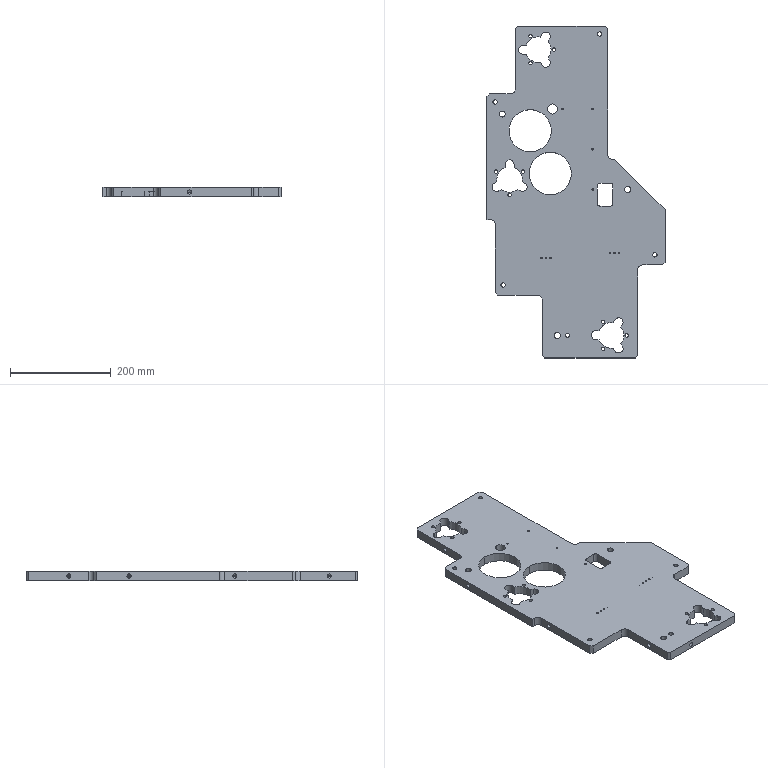NC program | NX | posted with a generic post | part box 354 x 660 x 18 mm
Lines 42 to 865 of 43361:
(ZLEVEL_PROFILE , TOOL : D8C)
N76 T08 M6
N78 G54
N80 G17 G0 G90 X-315.203 Y87.193 S4000 M3
N82 G43 Z30. H8
N84 Z1.7
N86 G94 G1 X-315.332 Y86.951 Z1.686 F1000.
N88 X-315.481 Y86.678 Z1.669
N90 X-315.628 Y86.323 Z1.649
N92 X-315.717 Y86.025 Z1.633
N94 X-315.721 Y86.017 Z1.632
N96 X-315.811 Y85.714 Z1.616
N98 X-315.919 Y85.036 Z1.58
N100 X-315.926 Y84.721 Z1.563
N102 X-315.934 Y84.411 Z1.547
N104 X-315.894 Y83.955 Z1.523
N106 X-315.811 Y83.504 Z1.499
N108 X-315.721 Y83.208 Z1.483
N110 X-315.681 Y83.081 Z1.476
N112 X-315.596 Y82.804 Z1.461
N114 X-315.465 Y82.499 Z1.443
N116 X-315.323 Y82.247 Z1.428
N118 X-314.989 Y81.708 Z1.395
N120 X-314.625 Y81.271 Z1.365
N122 X-314.42 Y81.044 Z1.349
N124 X-313.946 Y80.64 Z1.316
N126 X-313.679 Y80.469 Z1.3
N128 X-313.461 Y80.33 Z1.286
N130 X-313.463 Y80.327
N132 X-308.138 Y77.253 Z0.964
N134 X-307.891 Y77.111 Z0.949
N136 X-307.33 Y76.653 Z0.911
N138 X-306.858 Y76.104 Z0.873
N140 X-306.492 Y75.48 Z0.835
N142 X-306.242 Y74.8 Z0.797
N144 X-306.117 Y74.087 Z0.759
N146 X-306.12 Y73.363 Z0.721
N148 X-306.167 Y73.082 Z0.706
N150 X-306.273 Y72.404 Z0.67
N152 X-306.382 Y71.353 Z0.615
N154 X-306.444 Y70.298 Z0.56
N156 X-306.449 Y69.612 Z0.524
N158 X-306.445 Y68.931 Z0.488
N160 X-306.378 Y67.806 Z0.429
N162 X-306.256 Y66.685 Z0.37
N164 X-306.146 Y66.012 Z0.334
N166 X-306.143
N168 X-306.029 Y65.356 Z0.299
N170 X-305.915 Y64.834 Z0.271
N172 X-305.744 Y64.183 Z0.236
N174 X-305.673 Y63.879 Z0.219
N176 X-305.58 Y63.581 Z0.203
N178 X-305.487 Y63.285 Z0.187
N180 X-305.347 Y62.837 Z0.162
N182 X-305.35 Y62.828
N184 X-305.345 Y62.829
N186 X-305.305 Y62.696 Z0.154
N188 X-304.948 Y61.738 Z0.101
N190 X-304.951 Y61.732 Z0.1
N192 X-304.946 Y61.733
N194 X-304.549 Y60.8 F2500.
N196 X-304.195 Y60.044
N198 X-304.145 Y59.956
N200 X-303.751 Y59.207
N202 X-303.566 Y58.883
N204 G3 X-302.951 Y57.883 R13.689
N206 X-302.414 Y57.099 R14.8
N208 G1 X-302.149 Y56.737
N210 G3 X-301.638 Y56.085 R9.006
N212 X-300.947 Y55.275 R13.979
N214 X-299.794 Y54.088 R20.277
N216 X-298.914 Y53.295 R18.733
N218 G1 X-298.575 Y53.008
N220 X-297.741 Y52.352
N222 X-296.953 Y51.807
N224 G3 X-296.14 Y51.289 R12.608
N226 X-295.457 Y50.889 R6.805
N228 X-293.884 Y50.093 R16.957
N230 G1 X-293.643 Y49.967
N232 X-292.938 Y49.691
N234 X-292.463 Y49.497
N236 G2 X-289.95 Y45.751 R4.049
N238 G1 Y39.6
N240 G3 X-289.786 Y38.377 R5.145
N242 X-289.385 Y37.327 R4.407
N244 X-288.84 Y36.499 R5.438
N246 X-288.484 Y36.107 R2.892
N248 G1 X-288.478 Y36.1
N250 G3 X-287.61 Y35.408 R5.05
N252 G1 X-287.414 Y35.299
N254 G3 X-286.5 Y34.902 R4.509
N256 G1 X-286.489 Y34.895
N258 G3 X-283.504 Y34.898 R4.886
N260 G1 X-283.497 Y34.902
N262 G3 X-282.768 Y35.201 R4.285
N264 G1 X-282.572 Y35.303
N266 G3 X-281.522 Y36.096 R4.826
N268 G1 X-281.514 Y36.106
N270 G3 X-280.605 Y37.341 R4.982
N272 X-280.245 Y38.241 R5.914
N274 G1 X-280.209 Y38.39
N276 G3 X-280.052 Y39.6 R5.341
N278 G1 X-280.05
N280 Y45.756
N282 G2 X-277.425 Y49.542 R4.046
N284 G1 X-277.061 Y49.689
N286 X-276.448 Y49.934
N288 X-275.222 Y50.516
N290 X-274.216 Y51.069
N292 X-273.503 Y51.509
N294 G3 X-272.633 Y52.093 R13.692
N296 X-271.834 Y52.686 R11.162
N298 X-271.094 Y53.287 R12.577
N300 G1 X-270.87 Y53.482
N302 G3 X-267.85 Y56.737 R21.15
N304 G1 X-267.737 Y56.892
N306 X-267.351 Y57.421
N308 X-267.044 Y57.891
N310 G3 X-266.251 Y59.2 R19.575
N312 G1 X-266.246 Y59.199
N314 X-265.854 Y59.956
N316 X-265.684 Y60.268
N318 X-265.45 Y60.801
N320 X-265.412 Y60.886
N322 X-265.071 Y61.686
N324 X-265.051 Y61.74
N326 X-264.708 Y62.658
N328 X-264.652 Y62.838
N330 G3 X-264.253 Y64.19 R18.089
N332 X-263.857 Y66.001 R21.717
N334 G1 X-263.855 Y66.007
N336 G3 X-263.696 Y72.079 R21.95
N338 G1 X-263.849 Y73.202
N340 G2 X-261.866 Y77.251 R4.042
N342 G1 X-256.373 Y80.422
N344 X-256.312 Y80.474
N346 G3 X-255.145 Y81.532 R4.956
N348 G1 X-255.075 Y81.628
N350 G3 X-254.279 Y83.2 R5.039
N352 X-254.279 Y86.015 R4.902
N354 G1 X-254.283 Y86.019
N356 G3 X-254.677 Y86.974 R4.82
N358 G1 X-254.682 Y86.987
N360 G3 X-255.076 Y87.593 R5.023
N362 G1 X-255.081 Y87.594
N364 G3 X-255.3 Y87.871 R5.265
N366 G1 X-255.483 Y88.064
N368 G3 X-256.508 Y88.868 R4.695
N370 G1 X-256.728 Y88.989
N372 G3 X-257.377 Y89.273 R3.959
N374 X-260.678 Y89.274 R4.998
N376 G1 X-260.68 Y89.269
N378 G3 X-261.486 Y88.898 R5.067
N380 G1 X-261.487 Y88.901
N382 X-266.53 Y85.989
N384 X-266.88 Y85.794
N386 G2 X-271.38 Y86.182 R4.032
N388 G1 X-271.753 Y86.47
N390 X-272.302 Y86.905
N392 X-273.381 Y87.638
N394 X-274.293 Y88.197
N396 X-275.376 Y88.782
N398 X-275.578 Y88.874
N400 X-275.825 Y88.99
N402 G3 X-280.03 Y90.471 R20.692
N404 X-282.157 Y90.868 R23.522
N406 G1 X-282.164 Y90.872
N408 G3 X-282.971 Y90.956 R58.63
N410 X-287.321 Y90.926 R20.955
N412 G1 X-287.822 Y90.87
N414 X-287.834 Y90.872
N416 X-287.835 Y90.868
N418 G3 X-289.975 Y90.468 R22.685
N420 X-294.192 Y88.983 R21.031
N422 G1 X-294.431 Y88.869
N424 X-294.574 Y88.801
N426 X-295.2 Y88.469
N428 G3 X-295.91 Y88.071 R11.94
N430 G1 X-296.631 Y87.63
N432 X-297.719 Y86.89
N434 X-298.563 Y86.224
N436 X-298.763 Y86.071
N438 G2 X-303.18 Y85.822 R4.05
N440 G1 X-308.513 Y88.901
N442 G3 X-312.526 Y89.305 R4.979
N444 G1 X-312.633 Y89.267
N446 G3 X-313.324 Y88.963 R4.463
N448 G1 X-313.491 Y88.867
N450 G3 X-314.523 Y88.055 R4.659
N452 X-315.332 Y86.951 R4.692
N454 X-315.717 Y86.025 R4.823
N456 G1 X-315.721 Y86.017
N458 G3 X-315.926 Y84.721 R4.965
N460 X-315.721 Y83.208 R4.791
N462 G1 X-315.681 Y83.081
N464 G3 X-315.323 Y82.247 R4.196
N466 G1 X-314.989 Y81.708
N468 X-314.625 Y81.271
N470 G3 X-313.679 Y80.469 R4.668
N472 G1 X-313.461 Y80.33
N474 X-313.463 Y80.327
N476 X-308.138 Y77.253
N478 G2 X-306.167 Y73.082 R4.053
N480 G3 X-306.449 Y69.612 R23.545
N482 X-306.146 Y66.012 R23.225
N484 G1 X-306.143
N486 G3 X-305.744 Y64.183 R22.152
N488 X-305.58 Y63.581 R8.727
N490 G1 X-305.487 Y63.285
N492 X-305.347 Y62.837
N494 X-305.35 Y62.828
N496 X-305.345 Y62.829
N498 G3 X-305.257 Y62.566 R4.205
N500 G1 X-304.948 Y61.738
N502 X-304.951 Y61.732
N504 X-304.946 Y61.733
N506 X-304.951 Y61.732
N508 X-304.877 Y61.548 Z0.097
N510 X-304.802 Y61.365 Z0.093
N512 X-304.725 Y61.183 Z0.09
N514 X-304.647 Y61.002 Z0.086
N516 X-304.567 Y60.822 Z0.083
N518 X-304.485 Y60.642 Z0.079
N520 X-304.402 Y60.463 Z0.076
N522 X-304.317 Y60.284 Z0.072
N524 X-304.23 Y60.107 Z0.069
N526 X-304.142 Y59.93 Z0.066
N528 X-304.052 Y59.754 Z0.062
N530 X-303.96 Y59.579 Z0.059
N532 X-303.867 Y59.405 Z0.055
N534 X-303.772 Y59.232 Z0.052
N536 X-303.676 Y59.059 Z0.048
N538 X-303.578 Y58.888 Z0.045
N540 X-303.478 Y58.717 Z0.041
N542 X-303.377 Y58.547 Z0.038
N544 X-303.274 Y58.379 Z0.034
N546 X-303.17 Y58.211 Z0.031
N548 X-303.065 Y58.044 Z0.028
N550 X-302.957 Y57.878 Z0.024
N552 X-302.848 Y57.713 Z0.021
N554 X-302.738 Y57.549 Z0.017
N556 X-302.626 Y57.386 Z0.014
N558 X-302.513 Y57.225 Z0.01
N560 X-302.398 Y57.064 Z0.007
N562 X-302.282 Y56.904 Z0.003
N564 X-302.164 Y56.745 Z0.
N566 G3 X-292.571 Y49.54 R21.45
N568 G2 X-289.95 Y45.751 R4.05
N570 G1 Y39.61
N572 G3 X-285. Y34.66 R4.95
N574 X-280.05 Y39.61 R4.95
N576 G1 Y45.751
N578 G2 X-277.429 Y49.54 R4.05
N580 G3 X-263.834 Y73.088 R21.45
N582 G2 X-261.863 Y77.253 R4.05
N584 G1 X-256.544 Y80.323
N586 G3 X-254.732 Y87.085 R4.95
N588 X-261.494 Y88.897 R4.95
N590 G1 X-266.371 Y86.082
N592 X-266.551 Y85.977
N594 X-266.573 Y85.976
N596 G2 X-271.405 Y86.201 R4.05
N598 G3 X-298.166 Y86.544 R21.45
N600 G1 X-298.165 Y86.533
N602 X-298.444 Y86.318
N604 X-298.46 Y86.317
N606 G2 X-303.187 Y85.826 R4.05
N608 G1 X-308.506 Y88.897
N610 G3 X-315.268 Y87.085 R4.95
N612 X-313.456 Y80.323 R4.95
N614 G1 X-308.137 Y77.253
N616 G2 X-306.166 Y73.088 R4.05
N618 G3 X-304.951 Y61.732 R21.45
N620 G1 X-304.879 Y61.555 Z-0.003
N622 X-304.803 Y61.379 Z-0.007
N624 X-304.727 Y61.204 Z-0.01
N626 X-304.649 Y61.03 Z-0.013
N628 X-304.573 Y60.855 Z-0.017
N630 X-304.496 Y60.68 Z-0.02
N632 X-304.421 Y60.505 Z-0.023
N634 X-304.336 Y60.334 Z-0.027
N636 X-304.25 Y60.163 Z-0.03
N638 X-304.163 Y59.993 Z-0.033
N640 X-304.078 Y59.822 Z-0.037
N642 X-303.992 Y59.652 Z-0.04
N644 X-303.906 Y59.481 Z-0.043
N646 X-303.814 Y59.314 Z-0.047
N648 X-303.718 Y59.149 Z-0.05
N650 X-303.622 Y58.984 Z-0.053
N652 X-303.528 Y58.818 Z-0.057
N654 X-303.433 Y58.652 Z-0.06
N656 X-303.337 Y58.487 Z-0.063
N658 X-303.238 Y58.324 Z-0.067
N660 X-303.134 Y58.164 Z-0.07
N662 X-303.03 Y58.004 Z-0.073
N664 X-302.925 Y57.844 Z-0.077
N666 X-302.82 Y57.684 Z-0.08
N668 X-302.717 Y57.524 Z-0.083
N670 X-302.61 Y57.365 Z-0.087
N672 X-302.496 Y57.212 Z-0.09
N674 X-302.384 Y57.057 Z-0.093
N676 X-302.271 Y56.904 Z-0.097
N678 X-302.164 Y56.745 Z-0.1
N680 G3 X-292.571 Y49.54 R21.45
N682 G2 X-289.95 Y45.751 R4.05
N684 G1 Y39.61
N686 G3 X-285. Y34.66 R4.95
N688 X-280.05 Y39.61 R4.95
N690 G1 Y45.751
N692 G2 X-277.429 Y49.54 R4.05
N694 G3 X-263.834 Y73.088 R21.45
N696 G2 X-261.863 Y77.253 R4.05
N698 G1 X-256.544 Y80.323
N700 G3 X-254.732 Y87.085 R4.95
N702 X-261.494 Y88.897 R4.95
N704 G1 X-266.371 Y86.082
N706 X-266.551 Y85.977
N708 X-266.573 Y85.976
N710 G2 X-271.405 Y86.201 R4.05
N712 G3 X-298.166 Y86.544 R21.45
N714 G1 X-298.165 Y86.533
N716 X-298.444 Y86.318
N718 X-298.46 Y86.317
N720 G2 X-303.187 Y85.826 R4.05
N722 G1 X-308.506 Y88.897
N724 G3 X-315.268 Y87.085 R4.95
N726 X-313.456 Y80.323 R4.95
N728 G1 X-308.137 Y77.253
N730 G2 X-306.166 Y73.088 R4.05
N732 G3 X-304.951 Y61.732 R21.45
N734 G1 X-304.879 Y61.555 Z-0.103
N736 X-304.803 Y61.379 Z-0.107
N738 X-304.727 Y61.204 Z-0.11
N740 X-304.649 Y61.03 Z-0.113
N742 X-304.573 Y60.855 Z-0.117
N744 X-304.496 Y60.68 Z-0.12
N746 X-304.421 Y60.505 Z-0.123
N748 X-304.336 Y60.334 Z-0.127
N750 X-304.25 Y60.163 Z-0.13
N752 X-304.163 Y59.993 Z-0.133
N754 X-304.078 Y59.822 Z-0.137
N756 X-303.992 Y59.652 Z-0.14
N758 X-303.906 Y59.481 Z-0.143
N760 X-303.814 Y59.314 Z-0.147
N762 X-303.718 Y59.149 Z-0.15
N764 X-303.622 Y58.984 Z-0.153
N766 X-303.528 Y58.818 Z-0.157
N768 X-303.433 Y58.652 Z-0.16
N770 X-303.337 Y58.487 Z-0.163
N772 X-303.238 Y58.324 Z-0.167
N774 X-303.134 Y58.164 Z-0.17
N776 X-303.03 Y58.004 Z-0.173
N778 X-302.925 Y57.844 Z-0.177
N780 X-302.82 Y57.684 Z-0.18
N782 X-302.717 Y57.524 Z-0.183
N784 X-302.61 Y57.365 Z-0.187
N786 X-302.496 Y57.212 Z-0.19
N788 X-302.384 Y57.057 Z-0.193
N790 X-302.271 Y56.904 Z-0.197
N792 X-302.164 Y56.745 Z-0.2
N794 G3 X-292.571 Y49.54 R21.45
N796 G2 X-289.95 Y45.751 R4.05
N798 G1 Y39.61
N800 G3 X-285. Y34.66 R4.95
N802 X-280.05 Y39.61 R4.95
N804 G1 Y45.751
N806 G2 X-277.429 Y49.54 R4.05
N808 G3 X-263.834 Y73.088 R21.45
N810 G2 X-261.863 Y77.253 R4.05
N812 G1 X-256.544 Y80.323
N814 G3 X-254.732 Y87.085 R4.95
N816 X-261.494 Y88.897 R4.95
N818 G1 X-266.371 Y86.082
N820 X-266.551 Y85.977
N822 X-266.573 Y85.976
N824 G2 X-271.405 Y86.201 R4.05
N826 G3 X-298.166 Y86.544 R21.45
N828 G1 X-298.165 Y86.533
N830 X-298.444 Y86.318
N832 X-298.46 Y86.317
N834 G2 X-303.187 Y85.826 R4.05
N836 G1 X-308.506 Y88.897
N838 G3 X-315.268 Y87.085 R4.95
N840 X-313.456 Y80.323 R4.95
N842 G1 X-308.137 Y77.253
N844 G2 X-306.166 Y73.088 R4.05
N846 G3 X-304.951 Y61.732 R21.45
N848 G1 X-304.879 Y61.555 Z-0.203
N850 X-304.803 Y61.379 Z-0.207
N852 X-304.727 Y61.204 Z-0.21
N854 X-304.649 Y61.03 Z-0.213
N856 X-304.573 Y60.855 Z-0.217
N858 X-304.496 Y60.68 Z-0.22
N860 X-304.421 Y60.505 Z-0.223
N862 X-304.336 Y60.334 Z-0.227
N864 X-304.25 Y60.163 Z-0.23
N866 X-304.163 Y59.993 Z-0.233
N868 X-304.078 Y59.822 Z-0.237
N870 X-303.992 Y59.652 Z-0.24
N872 X-303.906 Y59.481 Z-0.243
N874 X-303.814 Y59.314 Z-0.247
N876 X-303.718 Y59.149 Z-0.25
N878 X-303.622 Y58.984 Z-0.253
N880 X-303.528 Y58.818 Z-0.257
N882 X-303.433 Y58.652 Z-0.26
N884 X-303.337 Y58.487 Z-0.263
N886 X-303.238 Y58.324 Z-0.267
N888 X-303.134 Y58.164 Z-0.27
N890 X-303.03 Y58.004 Z-0.273
N892 X-302.925 Y57.844 Z-0.277
N894 X-302.82 Y57.684 Z-0.28
N896 X-302.717 Y57.524 Z-0.283
N898 X-302.61 Y57.365 Z-0.287
N900 X-302.496 Y57.212 Z-0.29
N902 X-302.384 Y57.057 Z-0.293
N904 X-302.271 Y56.904 Z-0.297
N906 X-302.164 Y56.745 Z-0.3
N908 G3 X-292.571 Y49.54 R21.45
N910 G2 X-289.95 Y45.751 R4.05
N912 G1 Y39.61
N914 G3 X-285. Y34.66 R4.95
N916 X-280.05 Y39.61 R4.95
N918 G1 Y45.751
N920 G2 X-277.429 Y49.54 R4.05
N922 G3 X-263.834 Y73.088 R21.45
N924 G2 X-261.863 Y77.253 R4.05
N926 G1 X-256.544 Y80.323
N928 G3 X-254.732 Y87.085 R4.95
N930 X-261.494 Y88.897 R4.95
N932 G1 X-266.371 Y86.082
N934 X-266.551 Y85.977
N936 X-266.573 Y85.976
N938 G2 X-271.405 Y86.201 R4.05
N940 G3 X-298.166 Y86.544 R21.45
N942 G1 X-298.165 Y86.533
N944 X-298.444 Y86.318
N946 X-298.46 Y86.317
N948 G2 X-303.187 Y85.826 R4.05
N950 G1 X-308.506 Y88.897
N952 G3 X-315.268 Y87.085 R4.95
N954 X-313.456 Y80.323 R4.95
N956 G1 X-308.137 Y77.253
N958 G2 X-306.166 Y73.088 R4.05
N960 G3 X-304.951 Y61.732 R21.45
N962 G1 X-304.879 Y61.555 Z-0.303
N964 X-304.803 Y61.379 Z-0.307
N966 X-304.727 Y61.204 Z-0.31
N968 X-304.649 Y61.03 Z-0.313
N970 X-304.573 Y60.855 Z-0.317
N972 X-304.496 Y60.68 Z-0.32
N974 X-304.421 Y60.505 Z-0.323
N976 X-304.336 Y60.334 Z-0.327
N978 X-304.25 Y60.163 Z-0.33
N980 X-304.163 Y59.993 Z-0.333
N982 X-304.078 Y59.822 Z-0.337
N984 X-303.992 Y59.652 Z-0.34
N986 X-303.906 Y59.481 Z-0.343
N988 X-303.814 Y59.314 Z-0.347
N990 X-303.718 Y59.149 Z-0.35
N992 X-303.622 Y58.984 Z-0.353
N994 X-303.528 Y58.818 Z-0.357
N996 X-303.433 Y58.652 Z-0.36
N998 X-303.337 Y58.487 Z-0.363
N1000 X-303.238 Y58.324 Z-0.367
N1002 X-303.134 Y58.164 Z-0.37
N1004 X-303.03 Y58.004 Z-0.373
N1006 X-302.925 Y57.844 Z-0.377
N1008 X-302.82 Y57.684 Z-0.38
N1010 X-302.717 Y57.524 Z-0.383
N1012 X-302.61 Y57.365 Z-0.387
N1014 X-302.496 Y57.212 Z-0.39
N1016 X-302.384 Y57.057 Z-0.393
N1018 X-302.271 Y56.904 Z-0.397
N1020 X-302.164 Y56.745 Z-0.4
N1022 G3 X-292.571 Y49.54 R21.45
N1024 G2 X-289.95 Y45.751 R4.05
N1026 G1 Y39.61
N1028 G3 X-285. Y34.66 R4.95
N1030 X-280.05 Y39.61 R4.95
N1032 G1 Y45.751
N1034 G2 X-277.429 Y49.54 R4.05
N1036 G3 X-263.834 Y73.088 R21.45
N1038 G2 X-261.863 Y77.253 R4.05
N1040 G1 X-256.544 Y80.323
N1042 G3 X-254.732 Y87.085 R4.95
N1044 X-261.494 Y88.897 R4.95
N1046 G1 X-266.371 Y86.082
N1048 X-266.551 Y85.977
N1050 X-266.573 Y85.976
N1052 G2 X-271.405 Y86.201 R4.05
N1054 G3 X-298.166 Y86.544 R21.45
N1056 G1 X-298.165 Y86.533
N1058 X-298.444 Y86.318
N1060 X-298.46 Y86.317
N1062 G2 X-303.187 Y85.826 R4.05
N1064 G1 X-308.506 Y88.897
N1066 G3 X-315.268 Y87.085 R4.95
N1068 X-313.456 Y80.323 R4.95
N1070 G1 X-308.137 Y77.253
N1072 G2 X-306.166 Y73.088 R4.05
N1074 G3 X-304.951 Y61.732 R21.45
N1076 G1 X-304.879 Y61.555 Z-0.403
N1078 X-304.803 Y61.379 Z-0.407
N1080 X-304.727 Y61.204 Z-0.41
N1082 X-304.649 Y61.03 Z-0.413
N1084 X-304.573 Y60.855 Z-0.417
N1086 X-304.496 Y60.68 Z-0.42
N1088 X-304.421 Y60.505 Z-0.423
N1090 X-304.336 Y60.334 Z-0.427
N1092 X-304.25 Y60.163 Z-0.43
N1094 X-304.163 Y59.993 Z-0.433
N1096 X-304.078 Y59.822 Z-0.437
N1098 X-303.992 Y59.652 Z-0.44
N1100 X-303.906 Y59.481 Z-0.443
N1102 X-303.814 Y59.314 Z-0.447
N1104 X-303.718 Y59.149 Z-0.45
N1106 X-303.622 Y58.984 Z-0.453
N1108 X-303.528 Y58.818 Z-0.457
N1110 X-303.433 Y58.652 Z-0.46
N1112 X-303.337 Y58.487 Z-0.463
N1114 X-303.238 Y58.324 Z-0.467
N1116 X-303.134 Y58.164 Z-0.47
N1118 X-303.03 Y58.004 Z-0.473
N1120 X-302.925 Y57.844 Z-0.477
N1122 X-302.82 Y57.684 Z-0.48
N1124 X-302.717 Y57.524 Z-0.483
N1126 X-302.61 Y57.365 Z-0.487
N1128 X-302.496 Y57.212 Z-0.49
N1130 X-302.384 Y57.057 Z-0.493
N1132 X-302.271 Y56.904 Z-0.497
N1134 X-302.164 Y56.745 Z-0.5
N1136 G3 X-292.571 Y49.54 R21.45
N1138 G2 X-289.95 Y45.751 R4.05
N1140 G1 Y39.61
N1142 G3 X-285. Y34.66 R4.95
N1144 X-280.05 Y39.61 R4.95
N1146 G1 Y45.751
N1148 G2 X-277.429 Y49.54 R4.05
N1150 G3 X-263.834 Y73.088 R21.45
N1152 G2 X-261.863 Y77.253 R4.05
N1154 G1 X-256.544 Y80.323
N1156 G3 X-254.732 Y87.085 R4.95
N1158 X-261.494 Y88.897 R4.95
N1160 G1 X-266.371 Y86.082
N1162 X-266.551 Y85.977
N1164 X-266.573 Y85.976
N1166 G2 X-271.405 Y86.201 R4.05
N1168 G3 X-298.166 Y86.544 R21.45
N1170 G1 X-298.165 Y86.533
N1172 X-298.444 Y86.318
N1174 X-298.46 Y86.317
N1176 G2 X-303.187 Y85.826 R4.05
N1178 G1 X-308.506 Y88.897
N1180 G3 X-315.268 Y87.085 R4.95
N1182 X-313.456 Y80.323 R4.95
N1184 G1 X-308.137 Y77.253
N1186 G2 X-306.166 Y73.088 R4.05
N1188 G3 X-304.951 Y61.732 R21.45
N1190 G1 X-304.879 Y61.555 Z-0.503
N1192 X-304.803 Y61.379 Z-0.507
N1194 X-304.727 Y61.204 Z-0.51
N1196 X-304.649 Y61.03 Z-0.513
N1198 X-304.573 Y60.855 Z-0.517
N1200 X-304.496 Y60.68 Z-0.52
N1202 X-304.421 Y60.505 Z-0.523
N1204 X-304.336 Y60.334 Z-0.527
N1206 X-304.25 Y60.163 Z-0.53
N1208 X-304.163 Y59.993 Z-0.533
N1210 X-304.078 Y59.822 Z-0.537
N1212 X-303.992 Y59.652 Z-0.54
N1214 X-303.906 Y59.481 Z-0.543
N1216 X-303.814 Y59.314 Z-0.547
N1218 X-303.718 Y59.149 Z-0.55
N1220 X-303.622 Y58.984 Z-0.553
N1222 X-303.528 Y58.818 Z-0.557
N1224 X-303.433 Y58.652 Z-0.56
N1226 X-303.337 Y58.487 Z-0.563
N1228 X-303.238 Y58.324 Z-0.567
N1230 X-303.134 Y58.164 Z-0.57
N1232 X-303.03 Y58.004 Z-0.573
N1234 X-302.925 Y57.844 Z-0.577
N1236 X-302.82 Y57.684 Z-0.58
N1238 X-302.717 Y57.524 Z-0.583
N1240 X-302.61 Y57.365 Z-0.587
N1242 X-302.496 Y57.212 Z-0.59
N1244 X-302.384 Y57.057 Z-0.593
N1246 X-302.271 Y56.904 Z-0.597
N1248 X-302.164 Y56.745 Z-0.6
N1250 G3 X-292.571 Y49.54 R21.45
N1252 G2 X-289.95 Y45.751 R4.05
N1254 G1 Y39.61
N1256 G3 X-285. Y34.66 R4.95
N1258 X-280.05 Y39.61 R4.95
N1260 G1 Y45.751
N1262 G2 X-277.429 Y49.54 R4.05
N1264 G3 X-263.834 Y73.088 R21.45
N1266 G2 X-261.863 Y77.253 R4.05
N1268 G1 X-256.544 Y80.323
N1270 G3 X-254.732 Y87.085 R4.95
N1272 X-261.494 Y88.897 R4.95
N1274 G1 X-266.371 Y86.082
N1276 X-266.551 Y85.977
N1278 X-266.573 Y85.976
N1280 G2 X-271.405 Y86.201 R4.05
N1282 G3 X-298.166 Y86.544 R21.45
N1284 G1 X-298.165 Y86.533
N1286 X-298.444 Y86.318
N1288 X-298.46 Y86.317
N1290 G2 X-303.187 Y85.826 R4.05
N1292 G1 X-308.506 Y88.897
N1294 G3 X-315.268 Y87.085 R4.95
N1296 X-313.456 Y80.323 R4.95
N1298 G1 X-308.137 Y77.253
N1300 G2 X-306.166 Y73.088 R4.05
N1302 G3 X-304.951 Y61.732 R21.45
N1304 G1 X-304.879 Y61.555 Z-0.603
N1306 X-304.803 Y61.379 Z-0.607
N1308 X-304.727 Y61.204 Z-0.61
N1310 X-304.649 Y61.03 Z-0.613
N1312 X-304.573 Y60.855 Z-0.617
N1314 X-304.496 Y60.68 Z-0.62
N1316 X-304.421 Y60.505 Z-0.623
N1318 X-304.336 Y60.334 Z-0.627
N1320 X-304.25 Y60.163 Z-0.63
N1322 X-304.163 Y59.993 Z-0.633
N1324 X-304.078 Y59.822 Z-0.637
N1326 X-303.992 Y59.652 Z-0.64
N1328 X-303.906 Y59.481 Z-0.643
N1330 X-303.814 Y59.314 Z-0.647
N1332 X-303.718 Y59.149 Z-0.65
N1334 X-303.622 Y58.984 Z-0.653
N1336 X-303.528 Y58.818 Z-0.657
N1338 X-303.433 Y58.652 Z-0.66
N1340 X-303.337 Y58.487 Z-0.663
N1342 X-303.238 Y58.324 Z-0.667
N1344 X-303.134 Y58.164 Z-0.67
N1346 X-303.03 Y58.004 Z-0.673
N1348 X-302.925 Y57.844 Z-0.677
N1350 X-302.82 Y57.684 Z-0.68
N1352 X-302.717 Y57.524 Z-0.683
N1354 X-302.61 Y57.365 Z-0.687
N1356 X-302.496 Y57.212 Z-0.69
N1358 X-302.384 Y57.057 Z-0.693
N1360 X-302.271 Y56.904 Z-0.697
N1362 X-302.164 Y56.745 Z-0.7
N1364 G3 X-292.571 Y49.54 R21.45
N1366 G2 X-289.95 Y45.751 R4.05
N1368 G1 Y39.61
N1370 G3 X-285. Y34.66 R4.95
N1372 X-280.05 Y39.61 R4.95
N1374 G1 Y45.751
N1376 G2 X-277.429 Y49.54 R4.05
N1378 G3 X-263.834 Y73.088 R21.45
N1380 G2 X-261.863 Y77.253 R4.05
N1382 G1 X-256.544 Y80.323
N1384 G3 X-254.732 Y87.085 R4.95
N1386 X-261.494 Y88.897 R4.95
N1388 G1 X-266.371 Y86.082
N1390 X-266.551 Y85.977
N1392 X-266.573 Y85.976
N1394 G2 X-271.405 Y86.201 R4.05
N1396 G3 X-298.166 Y86.544 R21.45
N1398 G1 X-298.165 Y86.533
N1400 X-298.444 Y86.318
N1402 X-298.46 Y86.317
N1404 G2 X-303.187 Y85.826 R4.05
N1406 G1 X-308.506 Y88.897
N1408 G3 X-315.268 Y87.085 R4.95
N1410 X-313.456 Y80.323 R4.95
N1412 G1 X-308.137 Y77.253
N1414 G2 X-306.166 Y73.088 R4.05
N1416 G3 X-304.951 Y61.732 R21.45
N1418 G1 X-304.879 Y61.555 Z-0.703
N1420 X-304.803 Y61.379 Z-0.707
N1422 X-304.727 Y61.204 Z-0.71
N1424 X-304.649 Y61.03 Z-0.713
N1426 X-304.573 Y60.855 Z-0.717
N1428 X-304.496 Y60.68 Z-0.72
N1430 X-304.421 Y60.505 Z-0.723
N1432 X-304.336 Y60.334 Z-0.727
N1434 X-304.25 Y60.163 Z-0.73
N1436 X-304.163 Y59.993 Z-0.733
N1438 X-304.078 Y59.822 Z-0.737
N1440 X-303.992 Y59.652 Z-0.74
N1442 X-303.906 Y59.481 Z-0.743
N1444 X-303.814 Y59.314 Z-0.747
N1446 X-303.718 Y59.149 Z-0.75
N1448 X-303.622 Y58.984 Z-0.753
N1450 X-303.528 Y58.818 Z-0.757
N1452 X-303.433 Y58.652 Z-0.76
N1454 X-303.337 Y58.487 Z-0.763
N1456 X-303.238 Y58.324 Z-0.767
N1458 X-303.134 Y58.164 Z-0.77
N1460 X-303.03 Y58.004 Z-0.773
N1462 X-302.925 Y57.844 Z-0.777
N1464 X-302.82 Y57.684 Z-0.78
N1466 X-302.717 Y57.524 Z-0.783
N1468 X-302.61 Y57.365 Z-0.787
N1470 X-302.496 Y57.212 Z-0.79
N1472 X-302.384 Y57.057 Z-0.793
N1474 X-302.271 Y56.904 Z-0.797
N1476 X-302.164 Y56.745 Z-0.8
N1478 G3 X-292.571 Y49.54 R21.45
N1480 G2 X-289.95 Y45.751 R4.05
N1482 G1 Y39.61
N1484 G3 X-285. Y34.66 R4.95
N1486 X-280.05 Y39.61 R4.95
N1488 G1 Y45.751
N1490 G2 X-277.429 Y49.54 R4.05
N1492 G3 X-263.834 Y73.088 R21.45
N1494 G2 X-261.863 Y77.253 R4.05
N1496 G1 X-256.544 Y80.323
N1498 G3 X-254.732 Y87.085 R4.95
N1500 X-261.494 Y88.897 R4.95
N1502 G1 X-266.371 Y86.082
N1504 X-266.551 Y85.977
N1506 X-266.573 Y85.976
N1508 G2 X-271.405 Y86.201 R4.05
N1510 G3 X-298.166 Y86.544 R21.45
N1512 G1 X-298.165 Y86.533
N1514 X-298.444 Y86.318
N1516 X-298.46 Y86.317
N1518 G2 X-303.187 Y85.826 R4.05
N1520 G1 X-308.506 Y88.897
N1522 G3 X-315.268 Y87.085 R4.95
N1524 X-313.456 Y80.323 R4.95
N1526 G1 X-308.137 Y77.253
N1528 G2 X-306.166 Y73.088 R4.05
N1530 G3 X-304.951 Y61.732 R21.45
N1532 G1 X-304.879 Y61.555 Z-0.803
N1534 X-304.803 Y61.379 Z-0.807
N1536 X-304.727 Y61.204 Z-0.81
N1538 X-304.649 Y61.03 Z-0.813
N1540 X-304.573 Y60.855 Z-0.817
N1542 X-304.496 Y60.68 Z-0.82
N1544 X-304.421 Y60.505 Z-0.823
N1546 X-304.336 Y60.334 Z-0.827
N1548 X-304.25 Y60.163 Z-0.83
N1550 X-304.163 Y59.993 Z-0.833
N1552 X-304.078 Y59.822 Z-0.837
N1554 X-303.992 Y59.652 Z-0.84
N1556 X-303.906 Y59.481 Z-0.843
N1558 X-303.814 Y59.314 Z-0.847
N1560 X-303.718 Y59.149 Z-0.85
N1562 X-303.622 Y58.984 Z-0.853
N1564 X-303.528 Y58.818 Z-0.857
N1566 X-303.433 Y58.652 Z-0.86
N1568 X-303.337 Y58.487 Z-0.863
N1570 X-303.238 Y58.324 Z-0.867
N1572 X-303.134 Y58.164 Z-0.87
N1574 X-303.03 Y58.004 Z-0.873
N1576 X-302.925 Y57.844 Z-0.877
N1578 X-302.82 Y57.684 Z-0.88
N1580 X-302.717 Y57.524 Z-0.883
N1582 X-302.61 Y57.365 Z-0.887
N1584 X-302.496 Y57.212 Z-0.89
N1586 X-302.384 Y57.057 Z-0.893
N1588 X-302.271 Y56.904 Z-0.897
N1590 X-302.164 Y56.745 Z-0.9
N1592 G3 X-292.571 Y49.54 R21.45
N1594 G2 X-289.95 Y45.751 R4.05
N1596 G1 Y39.61
N1598 G3 X-285. Y34.66 R4.95
N1600 X-280.05 Y39.61 R4.95
N1602 G1 Y45.751
N1604 G2 X-277.429 Y49.54 R4.05
N1606 G3 X-263.834 Y73.088 R21.45
N1608 G2 X-261.863 Y77.253 R4.05
N1610 G1 X-256.544 Y80.323
N1612 G3 X-254.732 Y87.085 R4.95
N1614 X-261.494 Y88.897 R4.95
N1616 G1 X-266.371 Y86.082
N1618 X-266.551 Y85.977
N1620 X-266.573 Y85.976
N1622 G2 X-271.405 Y86.201 R4.05
N1624 G3 X-298.166 Y86.544 R21.45
N1626 G1 X-298.165 Y86.533
N1628 X-298.444 Y86.318
N1630 X-298.46 Y86.317
N1632 G2 X-303.187 Y85.826 R4.05
N1634 G1 X-308.506 Y88.897
N1636 G3 X-315.268 Y87.085 R4.95
N1638 X-313.456 Y80.323 R4.95
N1640 G1 X-308.137 Y77.253
N1642 G2 X-306.166 Y73.088 R4.05
N1644 G3 X-304.951 Y61.732 R21.45
N1646 G1 X-304.879 Y61.555 Z-0.903
N1648 X-304.803 Y61.379 Z-0.907
N1650 X-304.727 Y61.204 Z-0.91
N1652 X-304.649 Y61.03 Z-0.913
N1654 X-304.573 Y60.855 Z-0.917
N1656 X-304.496 Y60.68 Z-0.92
N1658 X-304.421 Y60.505 Z-0.923
N1660 X-304.336 Y60.334 Z-0.927
N1662 X-304.25 Y60.163 Z-0.93
N1664 X-304.163 Y59.993 Z-0.933
N1666 X-304.078 Y59.822 Z-0.937
N1668 X-303.992 Y59.652 Z-0.94
N1670 X-303.906 Y59.481 Z-0.943
N1672 X-303.814 Y59.314 Z-0.947
N1674 X-303.718 Y59.149 Z-0.95
N1676 X-303.622 Y58.984 Z-0.953
N1678 X-303.528 Y58.818 Z-0.957
N1680 X-303.433 Y58.652 Z-0.96
N1682 X-303.337 Y58.487 Z-0.963
N1684 X-303.238 Y58.324 Z-0.967
N1686 X-303.134 Y58.164 Z-0.97
N1688 X-303.03 Y58.004 Z-0.973
N1690 X-302.925 Y57.844 Z-0.977
N1692 X-302.82 Y57.684 Z-0.98
N1694 X-302.717 Y57.524 Z-0.983
N1696 X-302.61 Y57.365 Z-0.987
N1698 X-302.496 Y57.212 Z-0.99
N1700 X-302.384 Y57.057 Z-0.993
N1702 X-302.271 Y56.904 Z-0.997
N1704 X-302.164 Y56.745 Z-1.
N1706 G3 X-292.571 Y49.54 R21.45
N1708 G2 X-289.95 Y45.751 R4.05
N1710 G1 Y39.61
N1712 G3 X-285. Y34.66 R4.95
N1714 X-280.05 Y39.61 R4.95
N1716 G1 Y45.751